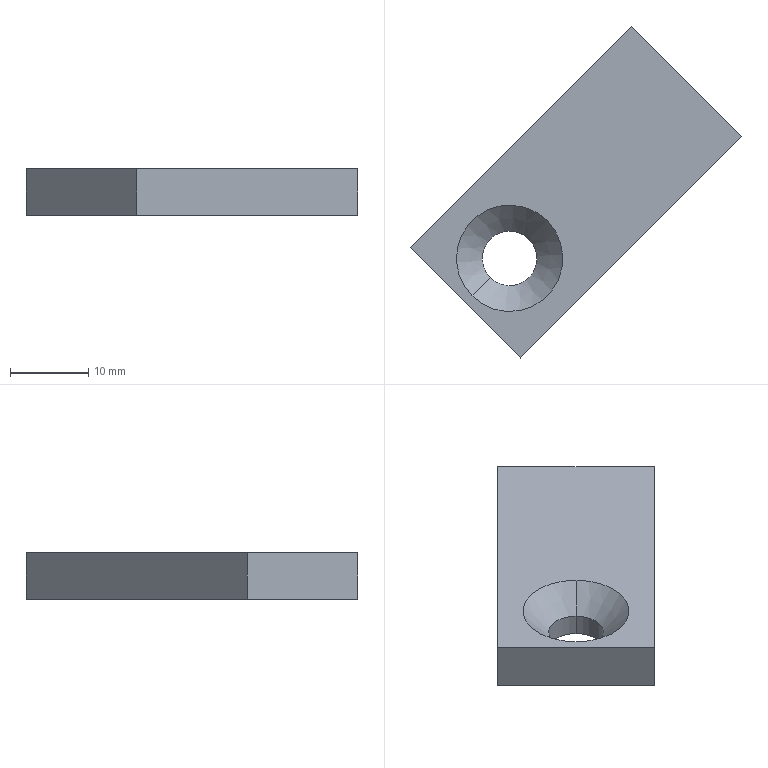Part | Creo | 1 solid | 10 faces | box 42.426 x 42.426 x 6 mm | volume 4412 mm3 | plane 6 | cone 2 | cylinder 2 | commonest cylinder face diameters 7 x2
STEP:
#1=CARTESIAN_POINT('',(-80.657,134.042,204.5));
#2=VERTEX_POINT('',#1);
#3=CARTESIAN_POINT('',(-66.515,119.899,204.5));
#4=VERTEX_POINT('',#3);
#5=CARTESIAN_POINT('',(-80.657,134.042,204.5));
#6=DIRECTION('',(0.7071,-0.7071,0.));
#7=VECTOR('',#6,20.);
#8=LINE('',#5,#7);
#9=EDGE_CURVE('',#2,#4,#8,.T.);
#10=ORIENTED_EDGE('',*,*,#9,.F.);
#11=CARTESIAN_POINT('',(-108.941,105.757,204.5));
#12=VERTEX_POINT('',#11);
#13=CARTESIAN_POINT('',(-108.941,105.757,204.5));
#14=DIRECTION('',(0.7071,0.7071,0.));
#15=VECTOR('',#14,40.);
#16=LINE('',#13,#15);
#17=EDGE_CURVE('',#12,#2,#16,.T.);
#18=ORIENTED_EDGE('',*,*,#17,.F.);
#19=CARTESIAN_POINT('',(-94.799,91.615,204.5));
#20=VERTEX_POINT('',#19);
#21=CARTESIAN_POINT('',(-94.799,91.615,204.5));
#22=DIRECTION('',(-0.7071,0.7071,0.));
#23=VECTOR('',#22,20.);
#24=LINE('',#21,#23);
#25=EDGE_CURVE('',#20,#12,#24,.T.);
#26=ORIENTED_EDGE('',*,*,#25,.F.);
#27=CARTESIAN_POINT('',(-66.515,119.899,204.5));
#28=DIRECTION('',(-0.7071,-0.7071,0.));
#29=VECTOR('',#28,40.);
#30=LINE('',#27,#29);
#31=EDGE_CURVE('',#4,#20,#30,.T.);
#32=ORIENTED_EDGE('',*,*,#31,.F.);
#33=EDGE_LOOP('',(#10,#18,#26,#32));
#34=FACE_OUTER_BOUND('',#33,.F.);
#35=CARTESIAN_POINT('',(-98.688,101.868,204.5));
#36=VERTEX_POINT('',#35);
#37=CARTESIAN_POINT('',(-93.738,106.818,204.5));
#38=VERTEX_POINT('',#37);
#39=CARTESIAN_POINT('',(-96.213,104.343,204.5));
#40=DIRECTION('',(0.,0.,1.));
#41=DIRECTION('',(-0.7071,-0.7071,0.));
#42=AXIS2_PLACEMENT_3D('',#39,#40,#41);
#43=CIRCLE('',#42,3.5);
#44=EDGE_CURVE('',#36,#38,#43,.T.);
#45=ORIENTED_EDGE('',*,*,#44,.F.);
#46=CARTESIAN_POINT('',(-96.213,104.343,204.5));
#47=DIRECTION('',(0.,0.,1.));
#48=DIRECTION('',(0.7071,0.7071,0.));
#49=AXIS2_PLACEMENT_3D('',#46,#47,#48);
#50=CIRCLE('',#49,3.5);
#51=EDGE_CURVE('',#38,#36,#50,.T.);
#52=ORIENTED_EDGE('',*,*,#51,.F.);
#53=EDGE_LOOP('',(#45,#52));
#54=FACE_BOUND('',#53,.F.);
#55=CARTESIAN_POINT('',(-87.728,112.828,204.5));
#56=DIRECTION('',(0.,0.,-1.));
#57=DIRECTION('',(-0.7071,-0.7071,0.));
#58=AXIS2_PLACEMENT_3D('',#55,#56,#57);
#59=PLANE('',#58);
#60=ADVANCED_FACE('',(#34,#54),#59,.T.);
#61=ORIENTED_EDGE('',*,*,#9,.T.);
#62=CARTESIAN_POINT('',(-66.515,119.899,210.5));
#63=VERTEX_POINT('',#62);
#64=CARTESIAN_POINT('',(-66.515,119.899,210.5));
#65=DIRECTION('',(0.,0.,-1.));
#66=VECTOR('',#65,6.);
#67=LINE('',#64,#66);
#68=EDGE_CURVE('',#63,#4,#67,.T.);
#69=ORIENTED_EDGE('',*,*,#68,.F.);
#70=CARTESIAN_POINT('',(-80.657,134.042,210.5));
#71=VERTEX_POINT('',#70);
#72=CARTESIAN_POINT('',(-66.515,119.899,210.5));
#73=DIRECTION('',(-0.7071,0.7071,0.));
#74=VECTOR('',#73,20.);
#75=LINE('',#72,#74);
#76=EDGE_CURVE('',#63,#71,#75,.T.);
#77=ORIENTED_EDGE('',*,*,#76,.T.);
#78=CARTESIAN_POINT('',(-80.657,134.042,210.5));
#79=DIRECTION('',(0.,0.,-1.));
#80=VECTOR('',#79,6.);
#81=LINE('',#78,#80);
#82=EDGE_CURVE('',#71,#2,#81,.T.);
#83=ORIENTED_EDGE('',*,*,#82,.T.);
#84=EDGE_LOOP('',(#61,#69,#77,#83));
#85=FACE_OUTER_BOUND('',#84,.F.);
#86=CARTESIAN_POINT('',(-73.586,126.971,204.5));
#87=DIRECTION('',(0.7071,0.7071,0.));
#88=DIRECTION('',(0.,0.,-1.));
#89=AXIS2_PLACEMENT_3D('',#86,#87,#88);
#90=PLANE('',#89);
#91=ADVANCED_FACE('',(#85),#90,.T.);
#92=ORIENTED_EDGE('',*,*,#68,.T.);
#93=ORIENTED_EDGE('',*,*,#31,.T.);
#94=CARTESIAN_POINT('',(-94.799,91.615,210.5));
#95=VERTEX_POINT('',#94);
#96=CARTESIAN_POINT('',(-94.799,91.615,210.5));
#97=DIRECTION('',(0.,0.,-1.));
#98=VECTOR('',#97,6.);
#99=LINE('',#96,#98);
#100=EDGE_CURVE('',#95,#20,#99,.T.);
#101=ORIENTED_EDGE('',*,*,#100,.F.);
#102=CARTESIAN_POINT('',(-94.799,91.615,210.5));
#103=DIRECTION('',(0.7071,0.7071,0.));
#104=VECTOR('',#103,40.);
#105=LINE('',#102,#104);
#106=EDGE_CURVE('',#95,#63,#105,.T.);
#107=ORIENTED_EDGE('',*,*,#106,.T.);
#108=EDGE_LOOP('',(#92,#93,#101,#107));
#109=FACE_OUTER_BOUND('',#108,.F.);
#110=CARTESIAN_POINT('',(-80.657,105.757,204.5));
#111=DIRECTION('',(0.7071,-0.7071,0.));
#112=DIRECTION('',(0.,0.,-1.));
#113=AXIS2_PLACEMENT_3D('',#110,#111,#112);
#114=PLANE('',#113);
#115=ADVANCED_FACE('',(#109),#114,.T.);
#116=ORIENTED_EDGE('',*,*,#100,.T.);
#117=ORIENTED_EDGE('',*,*,#25,.T.);
#118=CARTESIAN_POINT('',(-108.941,105.757,210.5));
#119=VERTEX_POINT('',#118);
#120=CARTESIAN_POINT('',(-108.941,105.757,210.5));
#121=DIRECTION('',(0.,0.,-1.));
#122=VECTOR('',#121,6.);
#123=LINE('',#120,#122);
#124=EDGE_CURVE('',#119,#12,#123,.T.);
#125=ORIENTED_EDGE('',*,*,#124,.F.);
#126=CARTESIAN_POINT('',(-108.941,105.757,210.5));
#127=DIRECTION('',(0.7071,-0.7071,0.));
#128=VECTOR('',#127,20.);
#129=LINE('',#126,#128);
#130=EDGE_CURVE('',#119,#95,#129,.T.);
#131=ORIENTED_EDGE('',*,*,#130,.T.);
#132=EDGE_LOOP('',(#116,#117,#125,#131));
#133=FACE_OUTER_BOUND('',#132,.F.);
#134=CARTESIAN_POINT('',(-101.87,98.686,204.5));
#135=DIRECTION('',(-0.7071,-0.7071,0.));
#136=DIRECTION('',(0.,0.,1.));
#137=AXIS2_PLACEMENT_3D('',#134,#135,#136);
#138=PLANE('',#137);
#139=ADVANCED_FACE('',(#133),#138,.T.);
#140=ORIENTED_EDGE('',*,*,#124,.T.);
#141=ORIENTED_EDGE('',*,*,#17,.T.);
#142=ORIENTED_EDGE('',*,*,#82,.F.);
#143=CARTESIAN_POINT('',(-80.657,134.042,210.5));
#144=DIRECTION('',(-0.7071,-0.7071,0.));
#145=VECTOR('',#144,40.);
#146=LINE('',#143,#145);
#147=EDGE_CURVE('',#71,#119,#146,.T.);
#148=ORIENTED_EDGE('',*,*,#147,.T.);
#149=EDGE_LOOP('',(#140,#141,#142,#148));
#150=FACE_OUTER_BOUND('',#149,.F.);
#151=CARTESIAN_POINT('',(-94.799,119.899,204.5));
#152=DIRECTION('',(-0.7071,0.7071,0.));
#153=DIRECTION('',(0.,0.,1.));
#154=AXIS2_PLACEMENT_3D('',#151,#152,#153);
#155=PLANE('',#154);
#156=ADVANCED_FACE('',(#150),#155,.T.);
#157=ORIENTED_EDGE('',*,*,#106,.F.);
#158=ORIENTED_EDGE('',*,*,#130,.F.);
#159=ORIENTED_EDGE('',*,*,#147,.F.);
#160=ORIENTED_EDGE('',*,*,#76,.F.);
#161=EDGE_LOOP('',(#157,#158,#159,#160));
#162=FACE_OUTER_BOUND('',#161,.F.);
#163=CARTESIAN_POINT('',(-91.405,109.151,210.5));
#164=VERTEX_POINT('',#163);
#165=CARTESIAN_POINT('',(-101.022,99.535,210.5));
#166=VERTEX_POINT('',#165);
#167=CARTESIAN_POINT('',(-96.213,104.343,210.5));
#168=DIRECTION('',(0.,0.,-1.));
#169=DIRECTION('',(0.7071,0.7071,0.));
#170=AXIS2_PLACEMENT_3D('',#167,#168,#169);
#171=CIRCLE('',#170,6.8);
#172=EDGE_CURVE('',#164,#166,#171,.T.);
#173=ORIENTED_EDGE('',*,*,#172,.F.);
#174=CARTESIAN_POINT('',(-96.213,104.343,210.5));
#175=DIRECTION('',(0.,0.,-1.));
#176=DIRECTION('',(-0.7071,-0.7071,0.));
#177=AXIS2_PLACEMENT_3D('',#174,#175,#176);
#178=CIRCLE('',#177,6.8);
#179=EDGE_CURVE('',#166,#164,#178,.T.);
#180=ORIENTED_EDGE('',*,*,#179,.F.);
#181=EDGE_LOOP('',(#173,#180));
#182=FACE_BOUND('',#181,.F.);
#183=CARTESIAN_POINT('',(-87.728,112.828,210.5));
#184=DIRECTION('',(0.,0.,1.));
#185=DIRECTION('',(0.7071,0.7071,0.));
#186=AXIS2_PLACEMENT_3D('',#183,#184,#185);
#187=PLANE('',#186);
#188=ADVANCED_FACE('',(#162,#182),#187,.T.);
#189=CARTESIAN_POINT('',(-93.738,106.818,207.2));
#190=VERTEX_POINT('',#189);
#191=CARTESIAN_POINT('',(-98.688,101.868,207.2));
#192=VERTEX_POINT('',#191);
#193=CARTESIAN_POINT('',(-96.213,104.343,207.2));
#194=DIRECTION('',(0.,0.,-1.));
#195=DIRECTION('',(0.7071,0.7071,0.));
#196=AXIS2_PLACEMENT_3D('',#193,#194,#195);
#197=CIRCLE('',#196,3.5);
#198=EDGE_CURVE('',#190,#192,#197,.T.);
#199=ORIENTED_EDGE('',*,*,#198,.F.);
#200=CARTESIAN_POINT('',(-93.738,106.818,207.2));
#201=DIRECTION('',(0.5,0.5,0.7071));
#202=VECTOR('',#201,4.667);
#203=LINE('',#200,#202);
#204=EDGE_CURVE('',#190,#164,#203,.T.);
#205=ORIENTED_EDGE('',*,*,#204,.T.);
#206=ORIENTED_EDGE('',*,*,#172,.T.);
#207=CARTESIAN_POINT('',(-98.688,101.868,207.2));
#208=DIRECTION('',(-0.5,-0.5,0.7071));
#209=VECTOR('',#208,4.667);
#210=LINE('',#207,#209);
#211=EDGE_CURVE('',#192,#166,#210,.T.);
#212=ORIENTED_EDGE('',*,*,#211,.F.);
#213=EDGE_LOOP('',(#199,#205,#206,#212));
#214=FACE_OUTER_BOUND('',#213,.F.);
#215=CARTESIAN_POINT('',(-96.213,104.343,208.85));
#216=DIRECTION('',(0.,0.,1.));
#217=DIRECTION('',(0.7071,0.7071,0.));
#218=AXIS2_PLACEMENT_3D('',#215,#216,#217);
#219=CONICAL_SURFACE('',#218,5.15,45.);
#220=ADVANCED_FACE('',(#214),#219,.F.);
#221=ORIENTED_EDGE('',*,*,#44,.T.);
#222=CARTESIAN_POINT('',(-93.738,106.818,204.5));
#223=DIRECTION('',(0.,0.,1.));
#224=VECTOR('',#223,2.7);
#225=LINE('',#222,#224);
#226=EDGE_CURVE('',#38,#190,#225,.T.);
#227=ORIENTED_EDGE('',*,*,#226,.T.);
#228=ORIENTED_EDGE('',*,*,#198,.T.);
#229=CARTESIAN_POINT('',(-98.688,101.868,204.5));
#230=DIRECTION('',(0.,0.,1.));
#231=VECTOR('',#230,2.7);
#232=LINE('',#229,#231);
#233=EDGE_CURVE('',#36,#192,#232,.T.);
#234=ORIENTED_EDGE('',*,*,#233,.F.);
#235=EDGE_LOOP('',(#221,#227,#228,#234));
#236=FACE_OUTER_BOUND('',#235,.F.);
#237=CARTESIAN_POINT('',(-96.213,104.343,210.307));
#238=DIRECTION('',(0.,0.,1.));
#239=DIRECTION('',(0.7071,0.7071,0.));
#240=AXIS2_PLACEMENT_3D('',#237,#238,#239);
#241=CYLINDRICAL_SURFACE('',#240,3.5);
#242=ADVANCED_FACE('',(#236),#241,.F.);
#243=ORIENTED_EDGE('',*,*,#51,.T.);
#244=ORIENTED_EDGE('',*,*,#233,.T.);
#245=CARTESIAN_POINT('',(-96.213,104.343,207.2));
#246=DIRECTION('',(0.,0.,-1.));
#247=DIRECTION('',(-0.7071,-0.7071,0.));
#248=AXIS2_PLACEMENT_3D('',#245,#246,#247);
#249=CIRCLE('',#248,3.5);
#250=EDGE_CURVE('',#192,#190,#249,.T.);
#251=ORIENTED_EDGE('',*,*,#250,.T.);
#252=ORIENTED_EDGE('',*,*,#226,.F.);
#253=EDGE_LOOP('',(#243,#244,#251,#252));
#254=FACE_OUTER_BOUND('',#253,.F.);
#255=CARTESIAN_POINT('',(-96.213,104.343,210.307));
#256=DIRECTION('',(0.,0.,1.));
#257=DIRECTION('',(0.7071,0.7071,0.));
#258=AXIS2_PLACEMENT_3D('',#255,#256,#257);
#259=CYLINDRICAL_SURFACE('',#258,3.5);
#260=ADVANCED_FACE('',(#254),#259,.F.);
#261=ORIENTED_EDGE('',*,*,#250,.F.);
#262=ORIENTED_EDGE('',*,*,#211,.T.);
#263=ORIENTED_EDGE('',*,*,#179,.T.);
#264=ORIENTED_EDGE('',*,*,#204,.F.);
#265=EDGE_LOOP('',(#261,#262,#263,#264));
#266=FACE_OUTER_BOUND('',#265,.F.);
#267=CARTESIAN_POINT('',(-96.213,104.343,208.85));
#268=DIRECTION('',(0.,0.,1.));
#269=DIRECTION('',(0.7071,0.7071,0.));
#270=AXIS2_PLACEMENT_3D('',#267,#268,#269);
#271=CONICAL_SURFACE('',#270,5.15,45.);
#272=ADVANCED_FACE('',(#266),#271,.F.);
#273=CLOSED_SHELL('',(#60,#91,#115,#139,#156,#188,#220,#242,#260,#272));
#274=MANIFOLD_SOLID_BREP('',#273);
#275=(LENGTH_UNIT()NAMED_UNIT(*)SI_UNIT(.MILLI.,.METRE.));
#276=UNCERTAINTY_MEASURE_WITH_UNIT(LENGTH_MEASURE(0.00603),#275,'','');
#277=(NAMED_UNIT(*)PLANE_ANGLE_UNIT()SI_UNIT($,.RADIAN.));
#278=PLANE_ANGLE_MEASURE_WITH_UNIT(PLANE_ANGLE_MEASURE(0.01745),#277);
#279=(CONVERSION_BASED_UNIT('DEGREE',#278)NAMED_UNIT(*)PLANE_ANGLE_UNIT());
#280=(NAMED_UNIT(*)SI_UNIT($,.STERADIAN.)SOLID_ANGLE_UNIT());
#281=(GEOMETRIC_REPRESENTATION_CONTEXT(3)GLOBAL_UNCERTAINTY_ASSIGNED_CONTEXT((#276))GLOBAL_UNIT_ASSIGNED_CONTEXT((#275,#279,#280))REPRESENTATION_CONTEXT('',''));
#282=ADVANCED_BREP_SHAPE_REPRESENTATION('',(#274),#281);